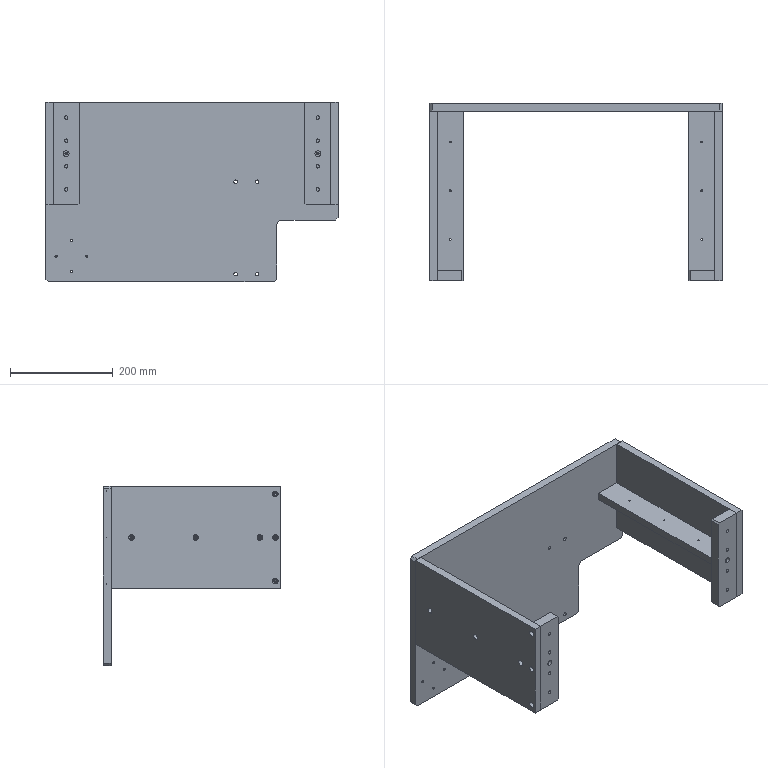Part | SolidWorks | 7 solids | 320 faces | box 570 x 345 x 350 mm | volume 5578892 mm3 | cylinder 193 | plane 83 | cone 44 | commonest cylinder face diameters 11 x60 6.6 x56 5 x32 5.2 x16 3.3 x12 4.2 x8